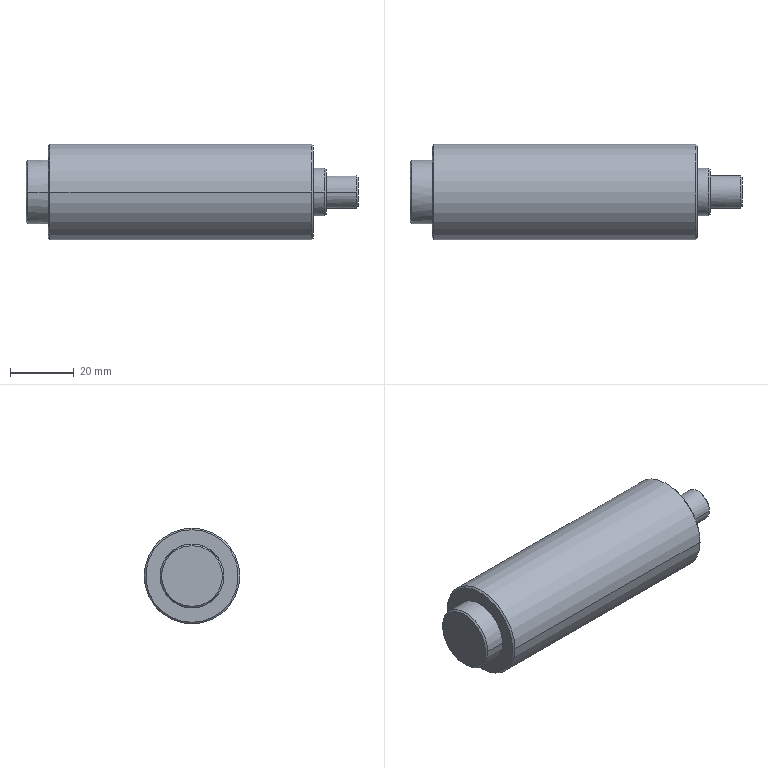Part | SolidWorks | features Chamfer 1, Revolution 1 | 1 solid | 23 faces | box 104 x 30 x 30 mm | volume 62360 mm3 | cone 10 | cylinder 8 | plane 5 | commonest cylinder face diameters 10.25 x2 15 x2 20 x2 30 x2
STEP:
#1=CARTESIAN_POINT('',(695.509,27.35,-4.625));
#2=VERTEX_POINT('',#1);
#3=CARTESIAN_POINT('',(695.509,27.35,4.625));
#4=VERTEX_POINT('',#3);
#5=CARTESIAN_POINT('',(695.509,27.35,0.));
#6=DIRECTION('',(1.,0.,0.));
#7=DIRECTION('',(0.,1.,0.));
#8=AXIS2_PLACEMENT_3D('',#5,#6,#7);
#9=CIRCLE('',#8,4.625);
#10=EDGE_CURVE('',#2,#4,#9,.T.);
#11=ORIENTED_EDGE('',*,*,#10,.F.);
#12=CARTESIAN_POINT('',(695.009,27.35,-5.125));
#13=VERTEX_POINT('',#12);
#14=CARTESIAN_POINT('',(695.509,27.35,-4.625));
#15=DIRECTION('',(-0.7071,0.,-0.7071));
#16=VECTOR('',#15,1000.);
#17=LINE('',#14,#16);
#18=EDGE_CURVE('',#2,#13,#17,.T.);
#19=ORIENTED_EDGE('',*,*,#18,.T.);
#20=CARTESIAN_POINT('',(695.009,32.475,0.));
#21=VERTEX_POINT('',#20);
#22=CARTESIAN_POINT('',(695.009,27.35,0.));
#23=DIRECTION('',(-1.,0.,0.));
#24=DIRECTION('',(0.,0.,-1.));
#25=AXIS2_PLACEMENT_3D('',#22,#23,#24);
#26=CIRCLE('',#25,5.125);
#27=EDGE_CURVE('',#21,#13,#26,.T.);
#28=ORIENTED_EDGE('',*,*,#27,.F.);
#29=CARTESIAN_POINT('',(695.009,27.35,5.125));
#30=VERTEX_POINT('',#29);
#31=CARTESIAN_POINT('',(695.009,27.35,0.));
#32=DIRECTION('',(-1.,0.,0.));
#33=DIRECTION('',(0.,0.,-1.));
#34=AXIS2_PLACEMENT_3D('',#31,#32,#33);
#35=CIRCLE('',#34,5.125);
#36=EDGE_CURVE('',#30,#21,#35,.T.);
#37=ORIENTED_EDGE('',*,*,#36,.F.);
#38=CARTESIAN_POINT('',(695.509,27.35,4.625));
#39=DIRECTION('',(-0.7071,0.,0.7071));
#40=VECTOR('',#39,1000.);
#41=LINE('',#38,#40);
#42=EDGE_CURVE('',#4,#30,#41,.T.);
#43=ORIENTED_EDGE('',*,*,#42,.F.);
#44=EDGE_LOOP('',(#11,#19,#28,#37,#43));
#45=FACE_OUTER_BOUND('',#44,.T.);
#46=CARTESIAN_POINT('',(695.509,27.35,0.));
#47=DIRECTION('',(-1.,0.,0.));
#48=DIRECTION('',(0.,0.,1.));
#49=AXIS2_PLACEMENT_3D('',#46,#47,#48);
#50=CONICAL_SURFACE('',#49,4.625,0.7854);
#51=ADVANCED_FACE('',(#45),#50,.T.);
#52=CARTESIAN_POINT('',(685.509,27.35,-7.));
#53=VERTEX_POINT('',#52);
#54=CARTESIAN_POINT('',(685.509,27.35,7.));
#55=VERTEX_POINT('',#54);
#56=CARTESIAN_POINT('',(685.509,27.35,0.));
#57=DIRECTION('',(1.,0.,0.));
#58=DIRECTION('',(0.,1.,0.));
#59=AXIS2_PLACEMENT_3D('',#56,#57,#58);
#60=CIRCLE('',#59,7.);
#61=EDGE_CURVE('',#53,#55,#60,.T.);
#62=ORIENTED_EDGE('',*,*,#61,.F.);
#63=CARTESIAN_POINT('',(685.009,27.35,-7.5));
#64=VERTEX_POINT('',#63);
#65=CARTESIAN_POINT('',(685.509,27.35,-7.));
#66=DIRECTION('',(-0.7071,0.,-0.7071));
#67=VECTOR('',#66,1000.);
#68=LINE('',#65,#67);
#69=EDGE_CURVE('',#53,#64,#68,.T.);
#70=ORIENTED_EDGE('',*,*,#69,.T.);
#71=CARTESIAN_POINT('',(685.009,34.85,0.));
#72=VERTEX_POINT('',#71);
#73=CARTESIAN_POINT('',(685.009,27.35,0.));
#74=DIRECTION('',(-1.,0.,0.));
#75=DIRECTION('',(0.,0.,-1.));
#76=AXIS2_PLACEMENT_3D('',#73,#74,#75);
#77=CIRCLE('',#76,7.5);
#78=EDGE_CURVE('',#72,#64,#77,.T.);
#79=ORIENTED_EDGE('',*,*,#78,.F.);
#80=CARTESIAN_POINT('',(685.009,27.35,7.5));
#81=VERTEX_POINT('',#80);
#82=CARTESIAN_POINT('',(685.009,27.35,0.));
#83=DIRECTION('',(-1.,0.,0.));
#84=DIRECTION('',(0.,0.,-1.));
#85=AXIS2_PLACEMENT_3D('',#82,#83,#84);
#86=CIRCLE('',#85,7.5);
#87=EDGE_CURVE('',#81,#72,#86,.T.);
#88=ORIENTED_EDGE('',*,*,#87,.F.);
#89=CARTESIAN_POINT('',(685.509,27.35,7.));
#90=DIRECTION('',(-0.7071,0.,0.7071));
#91=VECTOR('',#90,1000.);
#92=LINE('',#89,#91);
#93=EDGE_CURVE('',#55,#81,#92,.T.);
#94=ORIENTED_EDGE('',*,*,#93,.F.);
#95=EDGE_LOOP('',(#62,#70,#79,#88,#94));
#96=FACE_OUTER_BOUND('',#95,.T.);
#97=CARTESIAN_POINT('',(685.509,27.35,0.));
#98=DIRECTION('',(-1.,0.,0.));
#99=DIRECTION('',(0.,0.,1.));
#100=AXIS2_PLACEMENT_3D('',#97,#98,#99);
#101=CONICAL_SURFACE('',#100,7.,0.7854);
#102=ADVANCED_FACE('',(#96),#101,.T.);
#103=CARTESIAN_POINT('',(681.509,27.35,-14.5));
#104=VERTEX_POINT('',#103);
#105=CARTESIAN_POINT('',(681.509,27.35,14.5));
#106=VERTEX_POINT('',#105);
#107=CARTESIAN_POINT('',(681.509,27.35,0.));
#108=DIRECTION('',(1.,0.,0.));
#109=DIRECTION('',(0.,1.,0.));
#110=AXIS2_PLACEMENT_3D('',#107,#108,#109);
#111=CIRCLE('',#110,14.5);
#112=EDGE_CURVE('',#104,#106,#111,.T.);
#113=ORIENTED_EDGE('',*,*,#112,.F.);
#114=CARTESIAN_POINT('',(681.009,27.35,-15.));
#115=VERTEX_POINT('',#114);
#116=CARTESIAN_POINT('',(681.509,27.35,-14.5));
#117=DIRECTION('',(-0.7071,0.,-0.7071));
#118=VECTOR('',#117,1000.);
#119=LINE('',#116,#118);
#120=EDGE_CURVE('',#104,#115,#119,.T.);
#121=ORIENTED_EDGE('',*,*,#120,.T.);
#122=CARTESIAN_POINT('',(681.009,42.35,0.));
#123=VERTEX_POINT('',#122);
#124=CARTESIAN_POINT('',(681.009,27.35,0.));
#125=DIRECTION('',(-1.,0.,0.));
#126=DIRECTION('',(0.,0.,-1.));
#127=AXIS2_PLACEMENT_3D('',#124,#125,#126);
#128=CIRCLE('',#127,15.);
#129=EDGE_CURVE('',#123,#115,#128,.T.);
#130=ORIENTED_EDGE('',*,*,#129,.F.);
#131=CARTESIAN_POINT('',(681.009,27.35,15.));
#132=VERTEX_POINT('',#131);
#133=CARTESIAN_POINT('',(681.009,27.35,0.));
#134=DIRECTION('',(-1.,0.,0.));
#135=DIRECTION('',(0.,0.,-1.));
#136=AXIS2_PLACEMENT_3D('',#133,#134,#135);
#137=CIRCLE('',#136,15.);
#138=EDGE_CURVE('',#132,#123,#137,.T.);
#139=ORIENTED_EDGE('',*,*,#138,.F.);
#140=CARTESIAN_POINT('',(681.509,27.35,14.5));
#141=DIRECTION('',(-0.7071,0.,0.7071));
#142=VECTOR('',#141,1000.);
#143=LINE('',#140,#142);
#144=EDGE_CURVE('',#106,#132,#143,.T.);
#145=ORIENTED_EDGE('',*,*,#144,.F.);
#146=EDGE_LOOP('',(#113,#121,#130,#139,#145));
#147=FACE_OUTER_BOUND('',#146,.T.);
#148=CARTESIAN_POINT('',(681.509,27.35,0.));
#149=DIRECTION('',(-1.,0.,0.));
#150=DIRECTION('',(0.,0.,1.));
#151=AXIS2_PLACEMENT_3D('',#148,#149,#150);
#152=CONICAL_SURFACE('',#151,14.5,0.7854);
#153=ADVANCED_FACE('',(#147),#152,.T.);
#154=CARTESIAN_POINT('',(598.509,27.35,14.5));
#155=VERTEX_POINT('',#154);
#156=CARTESIAN_POINT('',(598.509,27.35,-14.5));
#157=VERTEX_POINT('',#156);
#158=CARTESIAN_POINT('',(598.509,27.35,0.));
#159=DIRECTION('',(-1.,0.,0.));
#160=DIRECTION('',(0.,-1.,0.));
#161=AXIS2_PLACEMENT_3D('',#158,#159,#160);
#162=CIRCLE('',#161,14.5);
#163=EDGE_CURVE('',#155,#157,#162,.T.);
#164=ORIENTED_EDGE('',*,*,#163,.F.);
#165=CARTESIAN_POINT('',(599.009,27.35,15.));
#166=VERTEX_POINT('',#165);
#167=CARTESIAN_POINT('',(599.009,27.35,15.));
#168=DIRECTION('',(0.7071,0.,0.7071));
#169=VECTOR('',#168,1000.);
#170=LINE('',#167,#169);
#171=EDGE_CURVE('',#155,#166,#170,.T.);
#172=ORIENTED_EDGE('',*,*,#171,.T.);
#173=CARTESIAN_POINT('',(599.009,42.35,0.));
#174=VERTEX_POINT('',#173);
#175=CARTESIAN_POINT('',(599.009,27.35,0.));
#176=DIRECTION('',(1.,0.,0.));
#177=DIRECTION('',(0.,0.,1.));
#178=AXIS2_PLACEMENT_3D('',#175,#176,#177);
#179=CIRCLE('',#178,15.);
#180=EDGE_CURVE('',#174,#166,#179,.T.);
#181=ORIENTED_EDGE('',*,*,#180,.F.);
#182=CARTESIAN_POINT('',(599.009,27.35,-15.));
#183=VERTEX_POINT('',#182);
#184=CARTESIAN_POINT('',(599.009,27.35,0.));
#185=DIRECTION('',(1.,0.,0.));
#186=DIRECTION('',(0.,0.,1.));
#187=AXIS2_PLACEMENT_3D('',#184,#185,#186);
#188=CIRCLE('',#187,15.);
#189=EDGE_CURVE('',#183,#174,#188,.T.);
#190=ORIENTED_EDGE('',*,*,#189,.F.);
#191=CARTESIAN_POINT('',(599.009,27.35,-15.));
#192=DIRECTION('',(0.7071,0.,-0.7071));
#193=VECTOR('',#192,1000.);
#194=LINE('',#191,#193);
#195=EDGE_CURVE('',#157,#183,#194,.T.);
#196=ORIENTED_EDGE('',*,*,#195,.F.);
#197=EDGE_LOOP('',(#164,#172,#181,#190,#196));
#198=FACE_OUTER_BOUND('',#197,.T.);
#199=CARTESIAN_POINT('',(599.009,27.35,0.));
#200=DIRECTION('',(1.,0.,0.));
#201=DIRECTION('',(0.,0.,-1.));
#202=AXIS2_PLACEMENT_3D('',#199,#200,#201);
#203=CONICAL_SURFACE('',#202,15.,0.7854);
#204=ADVANCED_FACE('',(#198),#203,.T.);
#205=CARTESIAN_POINT('',(591.509,27.35,9.5));
#206=VERTEX_POINT('',#205);
#207=CARTESIAN_POINT('',(591.509,27.35,-9.5));
#208=VERTEX_POINT('',#207);
#209=CARTESIAN_POINT('',(591.509,27.35,0.));
#210=DIRECTION('',(-1.,0.,0.));
#211=DIRECTION('',(0.,-1.,0.));
#212=AXIS2_PLACEMENT_3D('',#209,#210,#211);
#213=CIRCLE('',#212,9.5);
#214=EDGE_CURVE('',#206,#208,#213,.T.);
#215=ORIENTED_EDGE('',*,*,#214,.F.);
#216=CARTESIAN_POINT('',(592.009,27.35,10.));
#217=VERTEX_POINT('',#216);
#218=CARTESIAN_POINT('',(592.009,27.35,10.));
#219=DIRECTION('',(0.7071,0.,0.7071));
#220=VECTOR('',#219,1000.);
#221=LINE('',#218,#220);
#222=EDGE_CURVE('',#206,#217,#221,.T.);
#223=ORIENTED_EDGE('',*,*,#222,.T.);
#224=CARTESIAN_POINT('',(592.009,37.35,0.));
#225=VERTEX_POINT('',#224);
#226=CARTESIAN_POINT('',(592.009,27.35,0.));
#227=DIRECTION('',(1.,0.,0.));
#228=DIRECTION('',(0.,0.,1.));
#229=AXIS2_PLACEMENT_3D('',#226,#227,#228);
#230=CIRCLE('',#229,10.);
#231=EDGE_CURVE('',#225,#217,#230,.T.);
#232=ORIENTED_EDGE('',*,*,#231,.F.);
#233=CARTESIAN_POINT('',(592.009,27.35,-10.));
#234=VERTEX_POINT('',#233);
#235=CARTESIAN_POINT('',(592.009,27.35,0.));
#236=DIRECTION('',(1.,0.,0.));
#237=DIRECTION('',(0.,0.,1.));
#238=AXIS2_PLACEMENT_3D('',#235,#236,#237);
#239=CIRCLE('',#238,10.);
#240=EDGE_CURVE('',#234,#225,#239,.T.);
#241=ORIENTED_EDGE('',*,*,#240,.F.);
#242=CARTESIAN_POINT('',(592.009,27.35,-10.));
#243=DIRECTION('',(0.7071,0.,-0.7071));
#244=VECTOR('',#243,1000.);
#245=LINE('',#242,#244);
#246=EDGE_CURVE('',#208,#234,#245,.T.);
#247=ORIENTED_EDGE('',*,*,#246,.F.);
#248=EDGE_LOOP('',(#215,#223,#232,#241,#247));
#249=FACE_OUTER_BOUND('',#248,.T.);
#250=CARTESIAN_POINT('',(592.009,27.35,0.));
#251=DIRECTION('',(1.,0.,0.));
#252=DIRECTION('',(0.,0.,-1.));
#253=AXIS2_PLACEMENT_3D('',#250,#251,#252);
#254=CONICAL_SURFACE('',#253,10.,0.7854);
#255=ADVANCED_FACE('',(#249),#254,.T.);
#256=CARTESIAN_POINT('',(685.509,32.475,0.));
#257=VERTEX_POINT('',#256);
#258=CARTESIAN_POINT('',(685.509,22.225,0.));
#259=VERTEX_POINT('',#258);
#260=CARTESIAN_POINT('',(685.509,27.35,0.));
#261=DIRECTION('',(1.,0.,0.));
#262=DIRECTION('',(0.,1.,0.));
#263=AXIS2_PLACEMENT_3D('',#260,#261,#262);
#264=CIRCLE('',#263,5.125);
#265=EDGE_CURVE('',#257,#259,#264,.T.);
#266=ORIENTED_EDGE('',*,*,#265,.T.);
#267=CARTESIAN_POINT('',(695.009,22.225,0.));
#268=VERTEX_POINT('',#267);
#269=CARTESIAN_POINT('',(695.509,22.225,0.));
#270=DIRECTION('',(1.,0.,0.));
#271=VECTOR('',#270,1000.);
#272=LINE('',#269,#271);
#273=EDGE_CURVE('',#259,#268,#272,.T.);
#274=ORIENTED_EDGE('',*,*,#273,.T.);
#275=CARTESIAN_POINT('',(695.009,27.35,0.));
#276=DIRECTION('',(-1.,0.,0.));
#277=DIRECTION('',(0.,0.,-1.));
#278=AXIS2_PLACEMENT_3D('',#275,#276,#277);
#279=CIRCLE('',#278,5.125);
#280=EDGE_CURVE('',#268,#30,#279,.T.);
#281=ORIENTED_EDGE('',*,*,#280,.T.);
#282=ORIENTED_EDGE('',*,*,#36,.T.);
#283=CARTESIAN_POINT('',(695.509,32.475,0.));
#284=DIRECTION('',(1.,0.,0.));
#285=VECTOR('',#284,1000.);
#286=LINE('',#283,#285);
#287=EDGE_CURVE('',#257,#21,#286,.T.);
#288=ORIENTED_EDGE('',*,*,#287,.F.);
#289=EDGE_LOOP('',(#266,#274,#281,#282,#288));
#290=FACE_OUTER_BOUND('',#289,.T.);
#291=CARTESIAN_POINT('',(695.509,27.35,0.));
#292=DIRECTION('',(1.,0.,0.));
#293=DIRECTION('',(0.,1.,0.));
#294=AXIS2_PLACEMENT_3D('',#291,#292,#293);
#295=CYLINDRICAL_SURFACE('',#294,5.125);
#296=ADVANCED_FACE('',(#290),#295,.T.);
#297=CARTESIAN_POINT('',(681.509,34.85,0.));
#298=VERTEX_POINT('',#297);
#299=CARTESIAN_POINT('',(681.509,19.85,0.));
#300=VERTEX_POINT('',#299);
#301=CARTESIAN_POINT('',(681.509,27.35,0.));
#302=DIRECTION('',(1.,0.,0.));
#303=DIRECTION('',(0.,1.,0.));
#304=AXIS2_PLACEMENT_3D('',#301,#302,#303);
#305=CIRCLE('',#304,7.5);
#306=EDGE_CURVE('',#298,#300,#305,.T.);
#307=ORIENTED_EDGE('',*,*,#306,.T.);
#308=CARTESIAN_POINT('',(685.009,19.85,0.));
#309=VERTEX_POINT('',#308);
#310=CARTESIAN_POINT('',(695.509,19.85,0.));
#311=DIRECTION('',(1.,0.,0.));
#312=VECTOR('',#311,1000.);
#313=LINE('',#310,#312);
#314=EDGE_CURVE('',#300,#309,#313,.T.);
#315=ORIENTED_EDGE('',*,*,#314,.T.);
#316=CARTESIAN_POINT('',(685.009,27.35,0.));
#317=DIRECTION('',(-1.,0.,0.));
#318=DIRECTION('',(0.,0.,-1.));
#319=AXIS2_PLACEMENT_3D('',#316,#317,#318);
#320=CIRCLE('',#319,7.5);
#321=EDGE_CURVE('',#309,#81,#320,.T.);
#322=ORIENTED_EDGE('',*,*,#321,.T.);
#323=ORIENTED_EDGE('',*,*,#87,.T.);
#324=CARTESIAN_POINT('',(695.509,34.85,0.));
#325=DIRECTION('',(1.,0.,0.));
#326=VECTOR('',#325,1000.);
#327=LINE('',#324,#326);
#328=EDGE_CURVE('',#298,#72,#327,.T.);
#329=ORIENTED_EDGE('',*,*,#328,.F.);
#330=EDGE_LOOP('',(#307,#315,#322,#323,#329));
#331=FACE_OUTER_BOUND('',#330,.T.);
#332=CARTESIAN_POINT('',(695.509,27.35,0.));
#333=DIRECTION('',(1.,0.,0.));
#334=DIRECTION('',(0.,1.,0.));
#335=AXIS2_PLACEMENT_3D('',#332,#333,#334);
#336=CYLINDRICAL_SURFACE('',#335,7.5);
#337=ADVANCED_FACE('',(#331),#336,.T.);
#338=ORIENTED_EDGE('',*,*,#180,.T.);
#339=CARTESIAN_POINT('',(599.009,12.35,0.));
#340=VERTEX_POINT('',#339);
#341=CARTESIAN_POINT('',(599.009,27.35,0.));
#342=DIRECTION('',(1.,0.,0.));
#343=DIRECTION('',(0.,0.,1.));
#344=AXIS2_PLACEMENT_3D('',#341,#342,#343);
#345=CIRCLE('',#344,15.);
#346=EDGE_CURVE('',#166,#340,#345,.T.);
#347=ORIENTED_EDGE('',*,*,#346,.T.);
#348=CARTESIAN_POINT('',(681.009,12.35,0.));
#349=VERTEX_POINT('',#348);
#350=CARTESIAN_POINT('',(695.509,12.35,0.));
#351=DIRECTION('',(1.,0.,0.));
#352=VECTOR('',#351,1000.);
#353=LINE('',#350,#352);
#354=EDGE_CURVE('',#340,#349,#353,.T.);
#355=ORIENTED_EDGE('',*,*,#354,.T.);
#356=CARTESIAN_POINT('',(681.009,27.35,0.));
#357=DIRECTION('',(-1.,0.,0.));
#358=DIRECTION('',(0.,0.,-1.));
#359=AXIS2_PLACEMENT_3D('',#356,#357,#358);
#360=CIRCLE('',#359,15.);
#361=EDGE_CURVE('',#349,#132,#360,.T.);
#362=ORIENTED_EDGE('',*,*,#361,.T.);
#363=ORIENTED_EDGE('',*,*,#138,.T.);
#364=CARTESIAN_POINT('',(695.509,42.35,0.));
#365=DIRECTION('',(1.,0.,0.));
#366=VECTOR('',#365,1000.);
#367=LINE('',#364,#366);
#368=EDGE_CURVE('',#174,#123,#367,.T.);
#369=ORIENTED_EDGE('',*,*,#368,.F.);
#370=EDGE_LOOP('',(#338,#347,#355,#362,#363,#369));
#371=FACE_OUTER_BOUND('',#370,.T.);
#372=CARTESIAN_POINT('',(695.509,27.35,0.));
#373=DIRECTION('',(1.,0.,0.));
#374=DIRECTION('',(0.,1.,0.));
#375=AXIS2_PLACEMENT_3D('',#372,#373,#374);
#376=CYLINDRICAL_SURFACE('',#375,15.);
#377=ADVANCED_FACE('',(#371),#376,.T.);
#378=ORIENTED_EDGE('',*,*,#231,.T.);
#379=CARTESIAN_POINT('',(592.009,17.35,0.));
#380=VERTEX_POINT('',#379);
#381=CARTESIAN_POINT('',(592.009,27.35,0.));
#382=DIRECTION('',(1.,0.,0.));
#383=DIRECTION('',(0.,0.,1.));
#384=AXIS2_PLACEMENT_3D('',#381,#382,#383);
#385=CIRCLE('',#384,10.);
#386=EDGE_CURVE('',#217,#380,#385,.T.);
#387=ORIENTED_EDGE('',*,*,#386,.T.);
#388=CARTESIAN_POINT('',(598.509,17.35,0.));
#389=VERTEX_POINT('',#388);
#390=CARTESIAN_POINT('',(695.509,17.35,0.));
#391=DIRECTION('',(1.,0.,0.));
#392=VECTOR('',#391,1000.);
#393=LINE('',#390,#392);
#394=EDGE_CURVE('',#380,#389,#393,.T.);
#395=ORIENTED_EDGE('',*,*,#394,.T.);
#396=CARTESIAN_POINT('',(598.509,37.35,0.));
#397=VERTEX_POINT('',#396);
#398=CARTESIAN_POINT('',(598.509,27.35,0.));
#399=DIRECTION('',(1.,0.,0.));
#400=DIRECTION('',(0.,1.,0.));
#401=AXIS2_PLACEMENT_3D('',#398,#399,#400);
#402=CIRCLE('',#401,10.);
#403=EDGE_CURVE('',#397,#389,#402,.T.);
#404=ORIENTED_EDGE('',*,*,#403,.F.);
#405=CARTESIAN_POINT('',(695.509,37.35,0.));
#406=DIRECTION('',(1.,0.,0.));
#407=VECTOR('',#406,1000.);
#408=LINE('',#405,#407);
#409=EDGE_CURVE('',#225,#397,#408,.T.);
#410=ORIENTED_EDGE('',*,*,#409,.F.);
#411=EDGE_LOOP('',(#378,#387,#395,#404,#410));
#412=FACE_OUTER_BOUND('',#411,.T.);
#413=CARTESIAN_POINT('',(695.509,27.35,0.));
#414=DIRECTION('',(1.,0.,0.));
#415=DIRECTION('',(0.,1.,0.));
#416=AXIS2_PLACEMENT_3D('',#413,#414,#415);
#417=CYLINDRICAL_SURFACE('',#416,10.);
#418=ADVANCED_FACE('',(#412),#417,.T.);
#419=CARTESIAN_POINT('',(695.509,27.35,0.));
#420=DIRECTION('',(1.,0.,0.));
#421=DIRECTION('',(0.,1.,0.));
#422=AXIS2_PLACEMENT_3D('',#419,#420,#421);
#423=CIRCLE('',#422,4.625);
#424=EDGE_CURVE('',#4,#2,#423,.T.);
#425=ORIENTED_EDGE('',*,*,#424,.T.);
#426=ORIENTED_EDGE('',*,*,#10,.T.);
#427=EDGE_LOOP('',(#425,#426));
#428=FACE_OUTER_BOUND('',#427,.T.);
#429=CARTESIAN_POINT('',(695.509,32.475,0.));
#430=DIRECTION('',(1.,0.,0.));
#431=DIRECTION('',(0.,1.,0.));
#432=AXIS2_PLACEMENT_3D('',#429,#430,#431);
#433=PLANE('',#432);
#434=ADVANCED_FACE('',(#428),#433,.T.);
#435=CARTESIAN_POINT('',(591.509,27.35,0.));
#436=DIRECTION('',(-1.,0.,0.));
#437=DIRECTION('',(0.,-1.,0.));
#438=AXIS2_PLACEMENT_3D('',#435,#436,#437);
#439=CIRCLE('',#438,9.5);
#440=EDGE_CURVE('',#208,#206,#439,.T.);
#441=ORIENTED_EDGE('',*,*,#440,.T.);
#442=ORIENTED_EDGE('',*,*,#214,.T.);
#443=EDGE_LOOP('',(#441,#442));
#444=FACE_OUTER_BOUND('',#443,.T.);
#445=CARTESIAN_POINT('',(591.509,37.35,0.));
#446=DIRECTION('',(-1.,0.,0.));
#447=DIRECTION('',(0.,-1.,0.));
#448=AXIS2_PLACEMENT_3D('',#445,#446,#447);
#449=PLANE('',#448);
#450=ADVANCED_FACE('',(#444),#449,.T.);
#451=ORIENTED_EDGE('',*,*,#394,.F.);
#452=CARTESIAN_POINT('',(592.009,27.35,0.));
#453=DIRECTION('',(1.,0.,0.));
#454=DIRECTION('',(0.,0.,1.));
#455=AXIS2_PLACEMENT_3D('',#452,#453,#454);
#456=CIRCLE('',#455,10.);
#457=EDGE_CURVE('',#380,#234,#456,.T.);
#458=ORIENTED_EDGE('',*,*,#457,.T.);
#459=ORIENTED_EDGE('',*,*,#240,.T.);
#460=ORIENTED_EDGE('',*,*,#409,.T.);
#461=CARTESIAN_POINT('',(598.509,27.35,0.));
#462=DIRECTION('',(1.,0.,0.));
#463=DIRECTION('',(0.,1.,0.));
#464=AXIS2_PLACEMENT_3D('',#461,#462,#463);
#465=CIRCLE('',#464,10.);
#466=EDGE_CURVE('',#389,#397,#465,.T.);
#467=ORIENTED_EDGE('',*,*,#466,.F.);
#468=EDGE_LOOP('',(#451,#458,#459,#460,#467));
#469=FACE_OUTER_BOUND('',#468,.T.);
#470=CARTESIAN_POINT('',(695.509,27.35,0.));
#471=DIRECTION('',(1.,0.,0.));
#472=DIRECTION('',(0.,1.,0.));
#473=AXIS2_PLACEMENT_3D('',#470,#471,#472);
#474=CYLINDRICAL_SURFACE('',#473,10.);
#475=ADVANCED_FACE('',(#469),#474,.T.);
#476=CARTESIAN_POINT('',(598.509,27.35,0.));
#477=DIRECTION('',(-1.,0.,0.));
#478=DIRECTION('',(0.,-1.,0.));
#479=AXIS2_PLACEMENT_3D('',#476,#477,#478);
#480=CIRCLE('',#479,14.5);
#481=EDGE_CURVE('',#157,#155,#480,.T.);
#482=ORIENTED_EDGE('',*,*,#481,.T.);
#483=ORIENTED_EDGE('',*,*,#163,.T.);
#484=EDGE_LOOP('',(#482,#483));
#485=FACE_OUTER_BOUND('',#484,.T.);
#486=ORIENTED_EDGE('',*,*,#403,.T.);
#487=ORIENTED_EDGE('',*,*,#466,.T.);
#488=EDGE_LOOP('',(#486,#487));
#489=FACE_BOUND('',#488,.T.);
#490=CARTESIAN_POINT('',(598.509,42.35,0.));
#491=DIRECTION('',(-1.,0.,0.));
#492=DIRECTION('',(0.,-1.,0.));
#493=AXIS2_PLACEMENT_3D('',#490,#491,#492);
#494=PLANE('',#493);
#495=ADVANCED_FACE('',(#485,#489),#494,.T.);
#496=ORIENTED_EDGE('',*,*,#354,.F.);
#497=CARTESIAN_POINT('',(599.009,27.35,0.));
#498=DIRECTION('',(1.,0.,0.));
#499=DIRECTION('',(0.,0.,1.));
#500=AXIS2_PLACEMENT_3D('',#497,#498,#499);
#501=CIRCLE('',#500,15.);
#502=EDGE_CURVE('',#340,#183,#501,.T.);
#503=ORIENTED_EDGE('',*,*,#502,.T.);
#504=ORIENTED_EDGE('',*,*,#189,.T.);
#505=ORIENTED_EDGE('',*,*,#368,.T.);
#506=ORIENTED_EDGE('',*,*,#129,.T.);
#507=CARTESIAN_POINT('',(681.009,27.35,0.));
#508=DIRECTION('',(-1.,0.,0.));
#509=DIRECTION('',(0.,0.,-1.));
#510=AXIS2_PLACEMENT_3D('',#507,#508,#509);
#511=CIRCLE('',#510,15.);
#512=EDGE_CURVE('',#115,#349,#511,.T.);
#513=ORIENTED_EDGE('',*,*,#512,.T.);
#514=EDGE_LOOP('',(#496,#503,#504,#505,#506,#513));
#515=FACE_OUTER_BOUND('',#514,.T.);
#516=CARTESIAN_POINT('',(695.509,27.35,0.));
#517=DIRECTION('',(1.,0.,0.));
#518=DIRECTION('',(0.,1.,0.));
#519=AXIS2_PLACEMENT_3D('',#516,#517,#518);
#520=CYLINDRICAL_SURFACE('',#519,15.);
#521=ADVANCED_FACE('',(#515),#520,.T.);
#522=CARTESIAN_POINT('',(681.509,27.35,0.));
#523=DIRECTION('',(1.,0.,0.));
#524=DIRECTION('',(0.,1.,0.));
#525=AXIS2_PLACEMENT_3D('',#522,#523,#524);
#526=CIRCLE('',#525,14.5);
#527=EDGE_CURVE('',#106,#104,#526,.T.);
#528=ORIENTED_EDGE('',*,*,#527,.T.);
#529=ORIENTED_EDGE('',*,*,#112,.T.);
#530=EDGE_LOOP('',(#528,#529));
#531=FACE_OUTER_BOUND('',#530,.T.);
#532=ORIENTED_EDGE('',*,*,#306,.F.);
#533=CARTESIAN_POINT('',(681.509,27.35,0.));
#534=DIRECTION('',(1.,0.,0.));
#535=DIRECTION('',(0.,1.,0.));
#536=AXIS2_PLACEMENT_3D('',#533,#534,#535);
#537=CIRCLE('',#536,7.5);
#538=EDGE_CURVE('',#300,#298,#537,.T.);
#539=ORIENTED_EDGE('',*,*,#538,.F.);
#540=EDGE_LOOP('',(#532,#539));
#541=FACE_BOUND('',#540,.T.);
#542=CARTESIAN_POINT('',(681.509,34.85,0.));
#543=DIRECTION('',(1.,0.,0.));
#544=DIRECTION('',(0.,1.,0.));
#545=AXIS2_PLACEMENT_3D('',#542,#543,#544);
#546=PLANE('',#545);
#547=ADVANCED_FACE('',(#531,#541),#546,.T.);
#548=ORIENTED_EDGE('',*,*,#314,.F.);
#549=ORIENTED_EDGE('',*,*,#538,.T.);
#550=ORIENTED_EDGE('',*,*,#328,.T.);
#551=ORIENTED_EDGE('',*,*,#78,.T.);
#552=CARTESIAN_POINT('',(685.009,27.35,0.));
#553=DIRECTION('',(-1.,0.,0.));
#554=DIRECTION('',(0.,0.,-1.));
#555=AXIS2_PLACEMENT_3D('',#552,#553,#554);
#556=CIRCLE('',#555,7.5);
#557=EDGE_CURVE('',#64,#309,#556,.T.);
#558=ORIENTED_EDGE('',*,*,#557,.T.);
#559=EDGE_LOOP('',(#548,#549,#550,#551,#558));
#560=FACE_OUTER_BOUND('',#559,.T.);
#561=CARTESIAN_POINT('',(695.509,27.35,0.));
#562=DIRECTION('',(1.,0.,0.));
#563=DIRECTION('',(0.,1.,0.));
#564=AXIS2_PLACEMENT_3D('',#561,#562,#563);
#565=CYLINDRICAL_SURFACE('',#564,7.5);
#566=ADVANCED_FACE('',(#560),#565,.T.);
#567=CARTESIAN_POINT('',(685.509,27.35,0.));
#568=DIRECTION('',(1.,0.,0.));
#569=DIRECTION('',(0.,1.,0.));
#570=AXIS2_PLACEMENT_3D('',#567,#568,#569);
#571=CIRCLE('',#570,7.);
#572=EDGE_CURVE('',#55,#53,#571,.T.);
#573=ORIENTED_EDGE('',*,*,#572,.T.);
#574=ORIENTED_EDGE('',*,*,#61,.T.);
#575=EDGE_LOOP('',(#573,#574));
#576=FACE_OUTER_BOUND('',#575,.T.);
#577=ORIENTED_EDGE('',*,*,#265,.F.);
#578=CARTESIAN_POINT('',(685.509,27.35,0.));
#579=DIRECTION('',(1.,0.,0.));
#580=DIRECTION('',(0.,1.,0.));
#581=AXIS2_PLACEMENT_3D('',#578,#579,#580);
#582=CIRCLE('',#581,5.125);
#583=EDGE_CURVE('',#259,#257,#582,.T.);
#584=ORIENTED_EDGE('',*,*,#583,.F.);
#585=EDGE_LOOP('',(#577,#584));
#586=FACE_BOUND('',#585,.T.);
#587=CARTESIAN_POINT('',(685.509,32.475,0.));
#588=DIRECTION('',(1.,0.,0.));
#589=DIRECTION('',(0.,1.,0.));
#590=AXIS2_PLACEMENT_3D('',#587,#588,#589);
#591=PLANE('',#590);
#592=ADVANCED_FACE('',(#576,#586),#591,.T.);
#593=ORIENTED_EDGE('',*,*,#273,.F.);
#594=ORIENTED_EDGE('',*,*,#583,.T.);
#595=ORIENTED_EDGE('',*,*,#287,.T.);
#596=ORIENTED_EDGE('',*,*,#27,.T.);
#597=CARTESIAN_POINT('',(695.009,27.35,0.));
#598=DIRECTION('',(-1.,0.,0.));
#599=DIRECTION('',(0.,0.,-1.));
#600=AXIS2_PLACEMENT_3D('',#597,#598,#599);
#601=CIRCLE('',#600,5.125);
#602=EDGE_CURVE('',#13,#268,#601,.T.);
#603=ORIENTED_EDGE('',*,*,#602,.T.);
#604=EDGE_LOOP('',(#593,#594,#595,#596,#603));
#605=FACE_OUTER_BOUND('',#604,.T.);
#606=CARTESIAN_POINT('',(695.509,27.35,0.));
#607=DIRECTION('',(1.,0.,0.));
#608=DIRECTION('',(0.,1.,0.));
#609=AXIS2_PLACEMENT_3D('',#606,#607,#608);
#610=CYLINDRICAL_SURFACE('',#609,5.125);
#611=ADVANCED_FACE('',(#605),#610,.T.);
#612=ORIENTED_EDGE('',*,*,#222,.F.);
#613=ORIENTED_EDGE('',*,*,#440,.F.);
#614=ORIENTED_EDGE('',*,*,#246,.T.);
#615=ORIENTED_EDGE('',*,*,#457,.F.);
#616=ORIENTED_EDGE('',*,*,#386,.F.);
#617=EDGE_LOOP('',(#612,#613,#614,#615,#616));
#618=FACE_OUTER_BOUND('',#617,.T.);
#619=CARTESIAN_POINT('',(592.009,27.35,0.));
#620=DIRECTION('',(1.,0.,0.));
#621=DIRECTION('',(0.,0.,-1.));
#622=AXIS2_PLACEMENT_3D('',#619,#620,#621);
#623=CONICAL_SURFACE('',#622,10.,0.7854);
#624=ADVANCED_FACE('',(#618),#623,.T.);
#625=ORIENTED_EDGE('',*,*,#171,.F.);
#626=ORIENTED_EDGE('',*,*,#481,.F.);
#627=ORIENTED_EDGE('',*,*,#195,.T.);
#628=ORIENTED_EDGE('',*,*,#502,.F.);
#629=ORIENTED_EDGE('',*,*,#346,.F.);
#630=EDGE_LOOP('',(#625,#626,#627,#628,#629));
#631=FACE_OUTER_BOUND('',#630,.T.);
#632=CARTESIAN_POINT('',(599.009,27.35,0.));
#633=DIRECTION('',(1.,0.,0.));
#634=DIRECTION('',(0.,0.,-1.));
#635=AXIS2_PLACEMENT_3D('',#632,#633,#634);
#636=CONICAL_SURFACE('',#635,15.,0.7854);
#637=ADVANCED_FACE('',(#631),#636,.T.);
#638=ORIENTED_EDGE('',*,*,#120,.F.);
#639=ORIENTED_EDGE('',*,*,#527,.F.);
#640=ORIENTED_EDGE('',*,*,#144,.T.);
#641=ORIENTED_EDGE('',*,*,#361,.F.);
#642=ORIENTED_EDGE('',*,*,#512,.F.);
#643=EDGE_LOOP('',(#638,#639,#640,#641,#642));
#644=FACE_OUTER_BOUND('',#643,.T.);
#645=CARTESIAN_POINT('',(681.509,27.35,0.));
#646=DIRECTION('',(-1.,0.,0.));
#647=DIRECTION('',(0.,0.,1.));
#648=AXIS2_PLACEMENT_3D('',#645,#646,#647);
#649=CONICAL_SURFACE('',#648,14.5,0.7854);
#650=ADVANCED_FACE('',(#644),#649,.T.);
#651=ORIENTED_EDGE('',*,*,#69,.F.);
#652=ORIENTED_EDGE('',*,*,#572,.F.);
#653=ORIENTED_EDGE('',*,*,#93,.T.);
#654=ORIENTED_EDGE('',*,*,#321,.F.);
#655=ORIENTED_EDGE('',*,*,#557,.F.);
#656=EDGE_LOOP('',(#651,#652,#653,#654,#655));
#657=FACE_OUTER_BOUND('',#656,.T.);
#658=CARTESIAN_POINT('',(685.509,27.35,0.));
#659=DIRECTION('',(-1.,0.,0.));
#660=DIRECTION('',(0.,0.,1.));
#661=AXIS2_PLACEMENT_3D('',#658,#659,#660);
#662=CONICAL_SURFACE('',#661,7.,0.7854);
#663=ADVANCED_FACE('',(#657),#662,.T.);
#664=ORIENTED_EDGE('',*,*,#18,.F.);
#665=ORIENTED_EDGE('',*,*,#424,.F.);
#666=ORIENTED_EDGE('',*,*,#42,.T.);
#667=ORIENTED_EDGE('',*,*,#280,.F.);
#668=ORIENTED_EDGE('',*,*,#602,.F.);
#669=EDGE_LOOP('',(#664,#665,#666,#667,#668));
#670=FACE_OUTER_BOUND('',#669,.T.);
#671=CARTESIAN_POINT('',(695.509,27.35,0.));
#672=DIRECTION('',(-1.,0.,0.));
#673=DIRECTION('',(0.,0.,1.));
#674=AXIS2_PLACEMENT_3D('',#671,#672,#673);
#675=CONICAL_SURFACE('',#674,4.625,0.7854);
#676=ADVANCED_FACE('',(#670),#675,.T.);
#677=CLOSED_SHELL('',(#51,#102,#153,#204,#255,#296,#337,#377,#418,#434,#450,#475,#495,#521,#547,#566,#592,#611,#624,#637,#650,#663,#676));
#678=MANIFOLD_SOLID_BREP('',#677);
#679=CARTESIAN_POINT('',(0.,0.,0.));
#680=DIRECTION('',(0.,0.,1.));
#681=DIRECTION('',(1.,0.,0.));
#682=AXIS2_PLACEMENT_3D('',#679,#680,#681);
#683=(LENGTH_UNIT()NAMED_UNIT(*)SI_UNIT(.MILLI.,.METRE.));
#684=UNCERTAINTY_MEASURE_WITH_UNIT(LENGTH_MEASURE(0.00001),#683,'','');
#685=(NAMED_UNIT(*)PLANE_ANGLE_UNIT()SI_UNIT($,.RADIAN.));
#686=(NAMED_UNIT(*)SI_UNIT($,.STERADIAN.)SOLID_ANGLE_UNIT());
#687=(GEOMETRIC_REPRESENTATION_CONTEXT(3)GLOBAL_UNCERTAINTY_ASSIGNED_CONTEXT((#684))GLOBAL_UNIT_ASSIGNED_CONTEXT((#683,#685,#686))REPRESENTATION_CONTEXT('',''));
#688=ADVANCED_BREP_SHAPE_REPRESENTATION('',(#678,#682),#687);